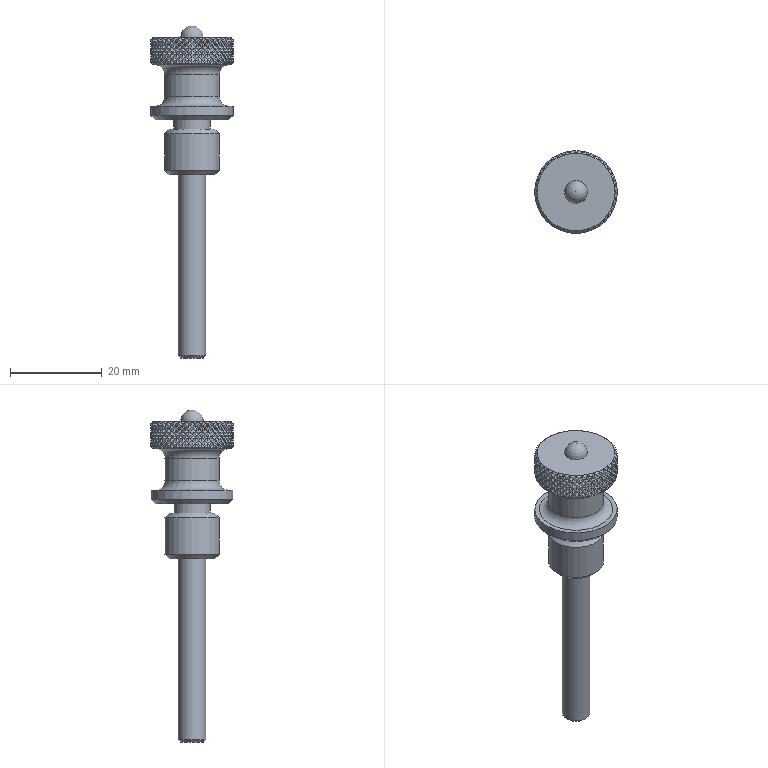Part | NX | features EXTRACT_STRING 82, SWP104 81, Instance Feature 79, DATUM_CSYS 4, CHAMFER 3, SKETCH 3, Pattern Feature 2, BLEND 1, DATUM_PLANE 1, Mirror Feature 1, WRAP 1 | 1 solid | 1941 faces | box 18 x 18 x 72.5 mm | volume 5643 mm3 | spline 1600 | cylinder 325 | plane 7 | cone 6 | torus 2 | sphere 1 | commonest cylinder face diameters 18 x321 12 x2 6 x1 8 x1